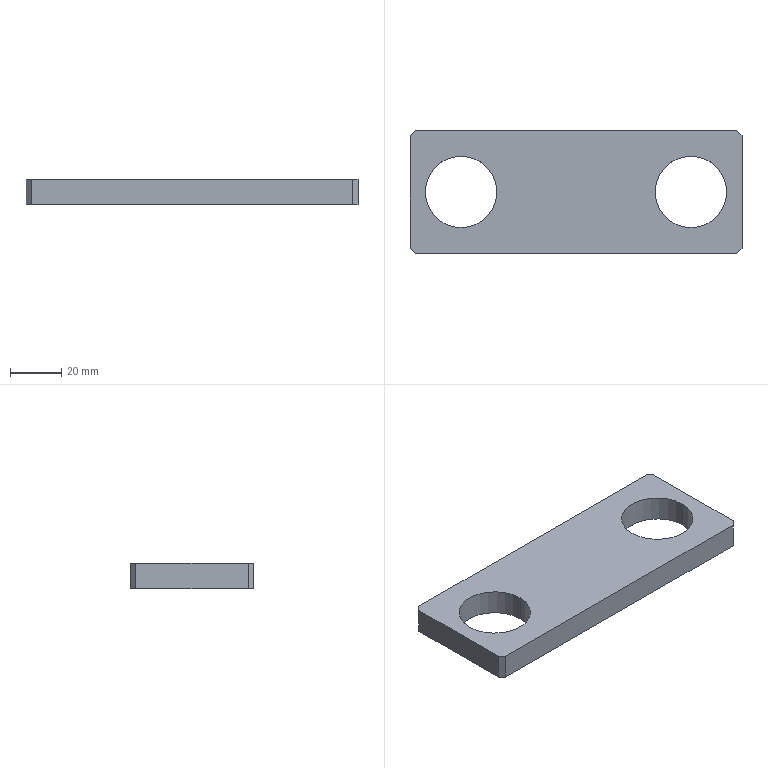Part | STEP file | Linear support fixing plate | 1 solid | 14 faces | box 130 x 48 x 10 mm | volume 50005 mm3 | plane 10 | cylinder 4 | commonest cylinder face diameters 28 x4
STEP:
#1=CARTESIAN_POINT('',(0.,0.,0.));
#2=DIRECTION('',(0.,0.,1.));
#3=DIRECTION('',(1.,0.,0.));
#4=AXIS2_PLACEMENT_3D('',#1,#2,#3);
#5=CARTESIAN_POINT('',(-31.,0.,0.));
#6=VERTEX_POINT('',#5);
#7=CARTESIAN_POINT('',(-31.,0.,10.));
#8=VERTEX_POINT('',#7);
#9=CARTESIAN_POINT('',(-31.,0.,0.));
#10=DIRECTION('',(0.,0.,1.));
#11=VECTOR('',#10,1.);
#12=LINE('',#9,#11);
#13=CARTESIAN_POINT('',(-45.,0.,0.));
#14=DIRECTION('',(0.,0.,1.));
#15=DIRECTION('',(1.,0.,0.));
#16=AXIS2_PLACEMENT_3D('',#13,#14,#15);
#17=CYLINDRICAL_SURFACE('',#16,14.);
#18=CARTESIAN_POINT('',(6.283,0.));
#19=DIRECTION('',(0.,1.));
#20=VECTOR('',#19,1.);
#21=LINE('',#18,#20);
#22=(GEOMETRIC_REPRESENTATION_CONTEXT(2)PARAMETRIC_REPRESENTATION_CONTEXT()REPRESENTATION_CONTEXT('',''));
#23=DEFINITIONAL_REPRESENTATION('',(#21),#22);
#24=PCURVE('',#17,#23);
#25=CARTESIAN_POINT('',(-45.,0.,0.));
#26=DIRECTION('',(0.,0.,1.));
#27=DIRECTION('',(1.,0.,0.));
#28=AXIS2_PLACEMENT_3D('',#25,#26,#27);
#29=CYLINDRICAL_SURFACE('',#28,14.);
#30=CARTESIAN_POINT('',(0.,0.));
#31=DIRECTION('',(0.,1.));
#32=VECTOR('',#31,1.);
#33=LINE('',#30,#32);
#34=(GEOMETRIC_REPRESENTATION_CONTEXT(2)PARAMETRIC_REPRESENTATION_CONTEXT()REPRESENTATION_CONTEXT('',''));
#35=DEFINITIONAL_REPRESENTATION('',(#33),#34);
#36=PCURVE('',#29,#35);
#37=SURFACE_CURVE('',#12,(#24,#36),.PCURVE_S1.);
#38=EDGE_CURVE('',#6,#8,#37,.T.);
#39=ORIENTED_EDGE('',*,*,#38,.T.);
#40=CARTESIAN_POINT('',(-59.,0.,10.));
#41=VERTEX_POINT('',#40);
#42=CARTESIAN_POINT('',(-45.,0.,10.));
#43=DIRECTION('',(0.,0.,-1.));
#44=DIRECTION('',(1.,0.,0.));
#45=AXIS2_PLACEMENT_3D('',#42,#43,#44);
#46=CIRCLE('',#45,14.);
#47=CARTESIAN_POINT('',(6.283,10.));
#48=DIRECTION('',(-1.,0.));
#49=VECTOR('',#48,1.);
#50=LINE('',#47,#49);
#51=(GEOMETRIC_REPRESENTATION_CONTEXT(2)PARAMETRIC_REPRESENTATION_CONTEXT()REPRESENTATION_CONTEXT('',''));
#52=DEFINITIONAL_REPRESENTATION('',(#50),#51);
#53=PCURVE('',#17,#52);
#54=CARTESIAN_POINT('',(0.,0.,10.));
#55=DIRECTION('',(0.,0.,1.));
#56=DIRECTION('',(1.,0.,0.));
#57=AXIS2_PLACEMENT_3D('',#54,#55,#56);
#58=PLANE('',#57);
#59=CARTESIAN_POINT('',(-31.,0.));
#60=CARTESIAN_POINT('',(-31.,-24.249));
#61=CARTESIAN_POINT('',(-52.,-12.124));
#62=CARTESIAN_POINT('',(-73.,0.));
#63=CARTESIAN_POINT('',(-52.,12.124));
#64=CARTESIAN_POINT('',(-31.,24.249));
#65=CARTESIAN_POINT('',(-31.,0.));
#66=(BOUNDED_CURVE()B_SPLINE_CURVE(2,(#59,#60,#61,#62,#63,#64,#65),.UNSPECIFIED.,.T.,.F.)B_SPLINE_CURVE_WITH_KNOTS((1,2,2,2,2,1),(-2.094,0.,2.094,4.189,6.283,8.378),.UNSPECIFIED.)CURVE()GEOMETRIC_REPRESENTATION_ITEM()RATIONAL_B_SPLINE_CURVE((1.,0.5,1.,0.5,1.,0.5,1.))REPRESENTATION_ITEM(''));
#67=(GEOMETRIC_REPRESENTATION_CONTEXT(2)PARAMETRIC_REPRESENTATION_CONTEXT()REPRESENTATION_CONTEXT('',''));
#68=DEFINITIONAL_REPRESENTATION('',(#66),#67);
#69=PCURVE('',#58,#68);
#70=SURFACE_CURVE('',#46,(#53,#69),.PCURVE_S1.);
#71=EDGE_CURVE('',#8,#41,#70,.T.);
#72=ORIENTED_EDGE('',*,*,#71,.T.);
#73=CARTESIAN_POINT('',(-59.,0.,0.));
#74=VERTEX_POINT('',#73);
#75=CARTESIAN_POINT('',(-59.,0.,0.));
#76=DIRECTION('',(0.,0.,1.));
#77=VECTOR('',#76,1.);
#78=LINE('',#75,#77);
#79=CARTESIAN_POINT('',(3.142,0.));
#80=DIRECTION('',(0.,1.));
#81=VECTOR('',#80,1.);
#82=LINE('',#79,#81);
#83=(GEOMETRIC_REPRESENTATION_CONTEXT(2)PARAMETRIC_REPRESENTATION_CONTEXT()REPRESENTATION_CONTEXT('',''));
#84=DEFINITIONAL_REPRESENTATION('',(#82),#83);
#85=PCURVE('',#17,#84);
#86=CARTESIAN_POINT('',(3.142,0.));
#87=DIRECTION('',(0.,1.));
#88=VECTOR('',#87,1.);
#89=LINE('',#86,#88);
#90=(GEOMETRIC_REPRESENTATION_CONTEXT(2)PARAMETRIC_REPRESENTATION_CONTEXT()REPRESENTATION_CONTEXT('',''));
#91=DEFINITIONAL_REPRESENTATION('',(#89),#90);
#92=PCURVE('',#29,#91);
#93=SURFACE_CURVE('',#78,(#85,#92),.PCURVE_S1.);
#94=EDGE_CURVE('',#74,#41,#93,.T.);
#95=ORIENTED_EDGE('',*,*,#94,.F.);
#96=CARTESIAN_POINT('',(-45.,0.,0.));
#97=DIRECTION('',(0.,0.,-1.));
#98=DIRECTION('',(1.,0.,0.));
#99=AXIS2_PLACEMENT_3D('',#96,#97,#98);
#100=CIRCLE('',#99,14.);
#101=CARTESIAN_POINT('',(6.283,0.));
#102=DIRECTION('',(-1.,0.));
#103=VECTOR('',#102,1.);
#104=LINE('',#101,#103);
#105=(GEOMETRIC_REPRESENTATION_CONTEXT(2)PARAMETRIC_REPRESENTATION_CONTEXT()REPRESENTATION_CONTEXT('',''));
#106=DEFINITIONAL_REPRESENTATION('',(#104),#105);
#107=PCURVE('',#17,#106);
#108=CARTESIAN_POINT('',(0.,0.,0.));
#109=DIRECTION('',(0.,0.,1.));
#110=DIRECTION('',(1.,0.,0.));
#111=AXIS2_PLACEMENT_3D('',#108,#109,#110);
#112=PLANE('',#111);
#113=CARTESIAN_POINT('',(-31.,0.));
#114=CARTESIAN_POINT('',(-31.,-24.249));
#115=CARTESIAN_POINT('',(-52.,-12.124));
#116=CARTESIAN_POINT('',(-73.,0.));
#117=CARTESIAN_POINT('',(-52.,12.124));
#118=CARTESIAN_POINT('',(-31.,24.249));
#119=CARTESIAN_POINT('',(-31.,0.));
#120=(BOUNDED_CURVE()B_SPLINE_CURVE(2,(#113,#114,#115,#116,#117,#118,#119),.UNSPECIFIED.,.T.,.F.)B_SPLINE_CURVE_WITH_KNOTS((1,2,2,2,2,1),(-2.094,0.,2.094,4.189,6.283,8.378),.UNSPECIFIED.)CURVE()GEOMETRIC_REPRESENTATION_ITEM()RATIONAL_B_SPLINE_CURVE((1.,0.5,1.,0.5,1.,0.5,1.))REPRESENTATION_ITEM(''));
#121=(GEOMETRIC_REPRESENTATION_CONTEXT(2)PARAMETRIC_REPRESENTATION_CONTEXT()REPRESENTATION_CONTEXT('',''));
#122=DEFINITIONAL_REPRESENTATION('',(#120),#121);
#123=PCURVE('',#112,#122);
#124=SURFACE_CURVE('',#100,(#107,#123),.PCURVE_S1.);
#125=EDGE_CURVE('',#6,#74,#124,.T.);
#126=ORIENTED_EDGE('',*,*,#125,.F.);
#127=EDGE_LOOP('',(#39,#72,#95,#126));
#128=FACE_BOUND('',#127,.F.);
#129=ADVANCED_FACE('',(#128),#17,.F.);
#130=CARTESIAN_POINT('',(59.,0.,0.));
#131=VERTEX_POINT('',#130);
#132=CARTESIAN_POINT('',(59.,0.,10.));
#133=VERTEX_POINT('',#132);
#134=CARTESIAN_POINT('',(59.,0.,0.));
#135=DIRECTION('',(0.,0.,1.));
#136=VECTOR('',#135,1.);
#137=LINE('',#134,#136);
#138=CARTESIAN_POINT('',(45.,0.,0.));
#139=DIRECTION('',(0.,0.,1.));
#140=DIRECTION('',(1.,0.,0.));
#141=AXIS2_PLACEMENT_3D('',#138,#139,#140);
#142=CYLINDRICAL_SURFACE('',#141,14.);
#143=CARTESIAN_POINT('',(6.283,0.));
#144=DIRECTION('',(0.,1.));
#145=VECTOR('',#144,1.);
#146=LINE('',#143,#145);
#147=(GEOMETRIC_REPRESENTATION_CONTEXT(2)PARAMETRIC_REPRESENTATION_CONTEXT()REPRESENTATION_CONTEXT('',''));
#148=DEFINITIONAL_REPRESENTATION('',(#146),#147);
#149=PCURVE('',#142,#148);
#150=CARTESIAN_POINT('',(45.,0.,0.));
#151=DIRECTION('',(0.,0.,1.));
#152=DIRECTION('',(1.,0.,0.));
#153=AXIS2_PLACEMENT_3D('',#150,#151,#152);
#154=CYLINDRICAL_SURFACE('',#153,14.);
#155=CARTESIAN_POINT('',(0.,0.));
#156=DIRECTION('',(0.,1.));
#157=VECTOR('',#156,1.);
#158=LINE('',#155,#157);
#159=(GEOMETRIC_REPRESENTATION_CONTEXT(2)PARAMETRIC_REPRESENTATION_CONTEXT()REPRESENTATION_CONTEXT('',''));
#160=DEFINITIONAL_REPRESENTATION('',(#158),#159);
#161=PCURVE('',#154,#160);
#162=SURFACE_CURVE('',#137,(#149,#161),.PCURVE_S1.);
#163=EDGE_CURVE('',#131,#133,#162,.T.);
#164=ORIENTED_EDGE('',*,*,#163,.T.);
#165=CARTESIAN_POINT('',(31.,0.,10.));
#166=VERTEX_POINT('',#165);
#167=CARTESIAN_POINT('',(45.,0.,10.));
#168=DIRECTION('',(0.,0.,-1.));
#169=DIRECTION('',(1.,0.,0.));
#170=AXIS2_PLACEMENT_3D('',#167,#168,#169);
#171=CIRCLE('',#170,14.);
#172=CARTESIAN_POINT('',(6.283,10.));
#173=DIRECTION('',(-1.,0.));
#174=VECTOR('',#173,1.);
#175=LINE('',#172,#174);
#176=(GEOMETRIC_REPRESENTATION_CONTEXT(2)PARAMETRIC_REPRESENTATION_CONTEXT()REPRESENTATION_CONTEXT('',''));
#177=DEFINITIONAL_REPRESENTATION('',(#175),#176);
#178=PCURVE('',#142,#177);
#179=CARTESIAN_POINT('',(59.,0.));
#180=CARTESIAN_POINT('',(59.,-24.249));
#181=CARTESIAN_POINT('',(38.,-12.124));
#182=CARTESIAN_POINT('',(17.,0.));
#183=CARTESIAN_POINT('',(38.,12.124));
#184=CARTESIAN_POINT('',(59.,24.249));
#185=CARTESIAN_POINT('',(59.,0.));
#186=(BOUNDED_CURVE()B_SPLINE_CURVE(2,(#179,#180,#181,#182,#183,#184,#185),.UNSPECIFIED.,.T.,.F.)B_SPLINE_CURVE_WITH_KNOTS((1,2,2,2,2,1),(-2.094,0.,2.094,4.189,6.283,8.378),.UNSPECIFIED.)CURVE()GEOMETRIC_REPRESENTATION_ITEM()RATIONAL_B_SPLINE_CURVE((1.,0.5,1.,0.5,1.,0.5,1.))REPRESENTATION_ITEM(''));
#187=(GEOMETRIC_REPRESENTATION_CONTEXT(2)PARAMETRIC_REPRESENTATION_CONTEXT()REPRESENTATION_CONTEXT('',''));
#188=DEFINITIONAL_REPRESENTATION('',(#186),#187);
#189=PCURVE('',#58,#188);
#190=SURFACE_CURVE('',#171,(#178,#189),.PCURVE_S1.);
#191=EDGE_CURVE('',#133,#166,#190,.T.);
#192=ORIENTED_EDGE('',*,*,#191,.T.);
#193=CARTESIAN_POINT('',(31.,0.,0.));
#194=VERTEX_POINT('',#193);
#195=CARTESIAN_POINT('',(31.,0.,0.));
#196=DIRECTION('',(0.,0.,1.));
#197=VECTOR('',#196,1.);
#198=LINE('',#195,#197);
#199=CARTESIAN_POINT('',(3.142,0.));
#200=DIRECTION('',(0.,1.));
#201=VECTOR('',#200,1.);
#202=LINE('',#199,#201);
#203=(GEOMETRIC_REPRESENTATION_CONTEXT(2)PARAMETRIC_REPRESENTATION_CONTEXT()REPRESENTATION_CONTEXT('',''));
#204=DEFINITIONAL_REPRESENTATION('',(#202),#203);
#205=PCURVE('',#142,#204);
#206=CARTESIAN_POINT('',(3.142,0.));
#207=DIRECTION('',(0.,1.));
#208=VECTOR('',#207,1.);
#209=LINE('',#206,#208);
#210=(GEOMETRIC_REPRESENTATION_CONTEXT(2)PARAMETRIC_REPRESENTATION_CONTEXT()REPRESENTATION_CONTEXT('',''));
#211=DEFINITIONAL_REPRESENTATION('',(#209),#210);
#212=PCURVE('',#154,#211);
#213=SURFACE_CURVE('',#198,(#205,#212),.PCURVE_S1.);
#214=EDGE_CURVE('',#194,#166,#213,.T.);
#215=ORIENTED_EDGE('',*,*,#214,.F.);
#216=CARTESIAN_POINT('',(45.,0.,0.));
#217=DIRECTION('',(0.,0.,-1.));
#218=DIRECTION('',(1.,0.,0.));
#219=AXIS2_PLACEMENT_3D('',#216,#217,#218);
#220=CIRCLE('',#219,14.);
#221=CARTESIAN_POINT('',(6.283,0.));
#222=DIRECTION('',(-1.,0.));
#223=VECTOR('',#222,1.);
#224=LINE('',#221,#223);
#225=(GEOMETRIC_REPRESENTATION_CONTEXT(2)PARAMETRIC_REPRESENTATION_CONTEXT()REPRESENTATION_CONTEXT('',''));
#226=DEFINITIONAL_REPRESENTATION('',(#224),#225);
#227=PCURVE('',#142,#226);
#228=CARTESIAN_POINT('',(59.,0.));
#229=CARTESIAN_POINT('',(59.,-24.249));
#230=CARTESIAN_POINT('',(38.,-12.124));
#231=CARTESIAN_POINT('',(17.,0.));
#232=CARTESIAN_POINT('',(38.,12.124));
#233=CARTESIAN_POINT('',(59.,24.249));
#234=CARTESIAN_POINT('',(59.,0.));
#235=(BOUNDED_CURVE()B_SPLINE_CURVE(2,(#228,#229,#230,#231,#232,#233,#234),.UNSPECIFIED.,.T.,.F.)B_SPLINE_CURVE_WITH_KNOTS((1,2,2,2,2,1),(-2.094,0.,2.094,4.189,6.283,8.378),.UNSPECIFIED.)CURVE()GEOMETRIC_REPRESENTATION_ITEM()RATIONAL_B_SPLINE_CURVE((1.,0.5,1.,0.5,1.,0.5,1.))REPRESENTATION_ITEM(''));
#236=(GEOMETRIC_REPRESENTATION_CONTEXT(2)PARAMETRIC_REPRESENTATION_CONTEXT()REPRESENTATION_CONTEXT('',''));
#237=DEFINITIONAL_REPRESENTATION('',(#235),#236);
#238=PCURVE('',#112,#237);
#239=SURFACE_CURVE('',#220,(#227,#238),.PCURVE_S1.);
#240=EDGE_CURVE('',#131,#194,#239,.T.);
#241=ORIENTED_EDGE('',*,*,#240,.F.);
#242=EDGE_LOOP('',(#164,#192,#215,#241));
#243=FACE_BOUND('',#242,.F.);
#244=ADVANCED_FACE('',(#243),#142,.F.);
#245=CARTESIAN_POINT('',(-63.,24.,0.));
#246=VERTEX_POINT('',#245);
#247=CARTESIAN_POINT('',(-65.,22.,0.));
#248=VERTEX_POINT('',#247);
#249=CARTESIAN_POINT('',(-63.,24.,0.));
#250=DIRECTION('',(-0.7071,-0.7071,0.));
#251=VECTOR('',#250,1.);
#252=LINE('',#249,#251);
#253=CARTESIAN_POINT('',(-63.,24.));
#254=DIRECTION('',(-0.7071,-0.7071));
#255=VECTOR('',#254,1.);
#256=LINE('',#253,#255);
#257=(GEOMETRIC_REPRESENTATION_CONTEXT(2)PARAMETRIC_REPRESENTATION_CONTEXT()REPRESENTATION_CONTEXT('',''));
#258=DEFINITIONAL_REPRESENTATION('',(#256),#257);
#259=PCURVE('',#112,#258);
#260=CARTESIAN_POINT('',(-65.,22.,10.));
#261=DIRECTION('',(0.7071,-0.7071,0.));
#262=DIRECTION('',(0.7071,0.7071,0.));
#263=AXIS2_PLACEMENT_3D('',#260,#261,#262);
#264=PLANE('',#263);
#265=CARTESIAN_POINT('',(2.828,-10.));
#266=DIRECTION('',(-1.,0.));
#267=VECTOR('',#266,1.);
#268=LINE('',#265,#267);
#269=(GEOMETRIC_REPRESENTATION_CONTEXT(2)PARAMETRIC_REPRESENTATION_CONTEXT()REPRESENTATION_CONTEXT('',''));
#270=DEFINITIONAL_REPRESENTATION('',(#268),#269);
#271=PCURVE('',#264,#270);
#272=SURFACE_CURVE('',#252,(#259,#271),.PCURVE_S1.);
#273=EDGE_CURVE('',#246,#248,#272,.T.);
#274=ORIENTED_EDGE('',*,*,#273,.F.);
#275=CARTESIAN_POINT('',(63.,24.,0.));
#276=VERTEX_POINT('',#275);
#277=CARTESIAN_POINT('',(0.,24.,0.));
#278=DIRECTION('',(-1.,0.,0.));
#279=VECTOR('',#278,1.);
#280=LINE('',#277,#279);
#281=CARTESIAN_POINT('',(0.,24.));
#282=DIRECTION('',(-1.,0.));
#283=VECTOR('',#282,1.);
#284=LINE('',#281,#283);
#285=(GEOMETRIC_REPRESENTATION_CONTEXT(2)PARAMETRIC_REPRESENTATION_CONTEXT()REPRESENTATION_CONTEXT('',''));
#286=DEFINITIONAL_REPRESENTATION('',(#284),#285);
#287=PCURVE('',#112,#286);
#288=CARTESIAN_POINT('',(-65.,24.,10.));
#289=DIRECTION('',(0.,-1.,0.));
#290=DIRECTION('',(0.,0.,-1.));
#291=AXIS2_PLACEMENT_3D('',#288,#289,#290);
#292=PLANE('',#291);
#293=CARTESIAN_POINT('',(10.,65.));
#294=DIRECTION('',(0.,-1.));
#295=VECTOR('',#294,1.);
#296=LINE('',#293,#295);
#297=(GEOMETRIC_REPRESENTATION_CONTEXT(2)PARAMETRIC_REPRESENTATION_CONTEXT()REPRESENTATION_CONTEXT('',''));
#298=DEFINITIONAL_REPRESENTATION('',(#296),#297);
#299=PCURVE('',#292,#298);
#300=SURFACE_CURVE('',#280,(#287,#299),.PCURVE_S1.);
#301=EDGE_CURVE('',#276,#246,#300,.T.);
#302=ORIENTED_EDGE('',*,*,#301,.F.);
#303=CARTESIAN_POINT('',(65.,22.,0.));
#304=VERTEX_POINT('',#303);
#305=CARTESIAN_POINT('',(65.,22.,0.));
#306=DIRECTION('',(-0.7071,0.7071,0.));
#307=VECTOR('',#306,1.);
#308=LINE('',#305,#307);
#309=CARTESIAN_POINT('',(65.,22.));
#310=DIRECTION('',(-0.7071,0.7071));
#311=VECTOR('',#310,1.);
#312=LINE('',#309,#311);
#313=(GEOMETRIC_REPRESENTATION_CONTEXT(2)PARAMETRIC_REPRESENTATION_CONTEXT()REPRESENTATION_CONTEXT('',''));
#314=DEFINITIONAL_REPRESENTATION('',(#312),#313);
#315=PCURVE('',#112,#314);
#316=CARTESIAN_POINT('',(63.,24.,10.));
#317=DIRECTION('',(-0.7071,-0.7071,0.));
#318=DIRECTION('',(0.7071,-0.7071,0.));
#319=AXIS2_PLACEMENT_3D('',#316,#317,#318);
#320=PLANE('',#319);
#321=CARTESIAN_POINT('',(2.828,-10.));
#322=DIRECTION('',(-1.,0.));
#323=VECTOR('',#322,1.);
#324=LINE('',#321,#323);
#325=(GEOMETRIC_REPRESENTATION_CONTEXT(2)PARAMETRIC_REPRESENTATION_CONTEXT()REPRESENTATION_CONTEXT('',''));
#326=DEFINITIONAL_REPRESENTATION('',(#324),#325);
#327=PCURVE('',#320,#326);
#328=SURFACE_CURVE('',#308,(#315,#327),.PCURVE_S1.);
#329=EDGE_CURVE('',#304,#276,#328,.T.);
#330=ORIENTED_EDGE('',*,*,#329,.F.);
#331=CARTESIAN_POINT('',(65.,-22.,0.));
#332=VERTEX_POINT('',#331);
#333=CARTESIAN_POINT('',(65.,0.,0.));
#334=DIRECTION('',(0.,1.,0.));
#335=VECTOR('',#334,1.);
#336=LINE('',#333,#335);
#337=CARTESIAN_POINT('',(65.,0.));
#338=DIRECTION('',(0.,1.));
#339=VECTOR('',#338,1.);
#340=LINE('',#337,#339);
#341=(GEOMETRIC_REPRESENTATION_CONTEXT(2)PARAMETRIC_REPRESENTATION_CONTEXT()REPRESENTATION_CONTEXT('',''));
#342=DEFINITIONAL_REPRESENTATION('',(#340),#341);
#343=PCURVE('',#112,#342);
#344=CARTESIAN_POINT('',(65.,24.,10.));
#345=DIRECTION('',(-1.,0.,0.));
#346=DIRECTION('',(0.,0.,1.));
#347=AXIS2_PLACEMENT_3D('',#344,#345,#346);
#348=PLANE('',#347);
#349=CARTESIAN_POINT('',(-10.,-24.));
#350=DIRECTION('',(0.,1.));
#351=VECTOR('',#350,1.);
#352=LINE('',#349,#351);
#353=(GEOMETRIC_REPRESENTATION_CONTEXT(2)PARAMETRIC_REPRESENTATION_CONTEXT()REPRESENTATION_CONTEXT('',''));
#354=DEFINITIONAL_REPRESENTATION('',(#352),#353);
#355=PCURVE('',#348,#354);
#356=SURFACE_CURVE('',#336,(#343,#355),.PCURVE_S1.);
#357=EDGE_CURVE('',#332,#304,#356,.T.);
#358=ORIENTED_EDGE('',*,*,#357,.F.);
#359=CARTESIAN_POINT('',(63.,-24.,0.));
#360=VERTEX_POINT('',#359);
#361=CARTESIAN_POINT('',(63.,-24.,0.));
#362=DIRECTION('',(0.7071,0.7071,0.));
#363=VECTOR('',#362,1.);
#364=LINE('',#361,#363);
#365=CARTESIAN_POINT('',(63.,-24.));
#366=DIRECTION('',(0.7071,0.7071));
#367=VECTOR('',#366,1.);
#368=LINE('',#365,#367);
#369=(GEOMETRIC_REPRESENTATION_CONTEXT(2)PARAMETRIC_REPRESENTATION_CONTEXT()REPRESENTATION_CONTEXT('',''));
#370=DEFINITIONAL_REPRESENTATION('',(#368),#369);
#371=PCURVE('',#112,#370);
#372=CARTESIAN_POINT('',(65.,-22.,10.));
#373=DIRECTION('',(-0.7071,0.7071,0.));
#374=DIRECTION('',(-0.7071,-0.7071,0.));
#375=AXIS2_PLACEMENT_3D('',#372,#373,#374);
#376=PLANE('',#375);
#377=CARTESIAN_POINT('',(2.828,-10.));
#378=DIRECTION('',(-1.,0.));
#379=VECTOR('',#378,1.);
#380=LINE('',#377,#379);
#381=(GEOMETRIC_REPRESENTATION_CONTEXT(2)PARAMETRIC_REPRESENTATION_CONTEXT()REPRESENTATION_CONTEXT('',''));
#382=DEFINITIONAL_REPRESENTATION('',(#380),#381);
#383=PCURVE('',#376,#382);
#384=SURFACE_CURVE('',#364,(#371,#383),.PCURVE_S1.);
#385=EDGE_CURVE('',#360,#332,#384,.T.);
#386=ORIENTED_EDGE('',*,*,#385,.F.);
#387=CARTESIAN_POINT('',(-63.,-24.,0.));
#388=VERTEX_POINT('',#387);
#389=CARTESIAN_POINT('',(0.,-24.,0.));
#390=DIRECTION('',(1.,0.,0.));
#391=VECTOR('',#390,1.);
#392=LINE('',#389,#391);
#393=CARTESIAN_POINT('',(0.,-24.));
#394=DIRECTION('',(1.,0.));
#395=VECTOR('',#394,1.);
#396=LINE('',#393,#395);
#397=(GEOMETRIC_REPRESENTATION_CONTEXT(2)PARAMETRIC_REPRESENTATION_CONTEXT()REPRESENTATION_CONTEXT('',''));
#398=DEFINITIONAL_REPRESENTATION('',(#396),#397);
#399=PCURVE('',#112,#398);
#400=CARTESIAN_POINT('',(-65.,-24.,10.));
#401=DIRECTION('',(0.,1.,0.));
#402=DIRECTION('',(0.,0.,1.));
#403=AXIS2_PLACEMENT_3D('',#400,#401,#402);
#404=PLANE('',#403);
#405=CARTESIAN_POINT('',(-10.,65.));
#406=DIRECTION('',(0.,1.));
#407=VECTOR('',#406,1.);
#408=LINE('',#405,#407);
#409=(GEOMETRIC_REPRESENTATION_CONTEXT(2)PARAMETRIC_REPRESENTATION_CONTEXT()REPRESENTATION_CONTEXT('',''));
#410=DEFINITIONAL_REPRESENTATION('',(#408),#409);
#411=PCURVE('',#404,#410);
#412=SURFACE_CURVE('',#392,(#399,#411),.PCURVE_S1.);
#413=EDGE_CURVE('',#388,#360,#412,.T.);
#414=ORIENTED_EDGE('',*,*,#413,.F.);
#415=CARTESIAN_POINT('',(-65.,-22.,0.));
#416=VERTEX_POINT('',#415);
#417=CARTESIAN_POINT('',(-65.,-22.,0.));
#418=DIRECTION('',(0.7071,-0.7071,0.));
#419=VECTOR('',#418,1.);
#420=LINE('',#417,#419);
#421=CARTESIAN_POINT('',(-65.,-22.));
#422=DIRECTION('',(0.7071,-0.7071));
#423=VECTOR('',#422,1.);
#424=LINE('',#421,#423);
#425=(GEOMETRIC_REPRESENTATION_CONTEXT(2)PARAMETRIC_REPRESENTATION_CONTEXT()REPRESENTATION_CONTEXT('',''));
#426=DEFINITIONAL_REPRESENTATION('',(#424),#425);
#427=PCURVE('',#112,#426);
#428=CARTESIAN_POINT('',(-63.,-24.,10.));
#429=DIRECTION('',(0.7071,0.7071,0.));
#430=DIRECTION('',(-0.7071,0.7071,0.));
#431=AXIS2_PLACEMENT_3D('',#428,#429,#430);
#432=PLANE('',#431);
#433=CARTESIAN_POINT('',(2.828,-10.));
#434=DIRECTION('',(-1.,0.));
#435=VECTOR('',#434,1.);
#436=LINE('',#433,#435);
#437=(GEOMETRIC_REPRESENTATION_CONTEXT(2)PARAMETRIC_REPRESENTATION_CONTEXT()REPRESENTATION_CONTEXT('',''));
#438=DEFINITIONAL_REPRESENTATION('',(#436),#437);
#439=PCURVE('',#432,#438);
#440=SURFACE_CURVE('',#420,(#427,#439),.PCURVE_S1.);
#441=EDGE_CURVE('',#416,#388,#440,.T.);
#442=ORIENTED_EDGE('',*,*,#441,.F.);
#443=CARTESIAN_POINT('',(-65.,0.,0.));
#444=DIRECTION('',(0.,-1.,0.));
#445=VECTOR('',#444,1.);
#446=LINE('',#443,#445);
#447=CARTESIAN_POINT('',(-65.,0.));
#448=DIRECTION('',(0.,-1.));
#449=VECTOR('',#448,1.);
#450=LINE('',#447,#449);
#451=(GEOMETRIC_REPRESENTATION_CONTEXT(2)PARAMETRIC_REPRESENTATION_CONTEXT()REPRESENTATION_CONTEXT('',''));
#452=DEFINITIONAL_REPRESENTATION('',(#450),#451);
#453=PCURVE('',#112,#452);
#454=CARTESIAN_POINT('',(-65.,24.,10.));
#455=DIRECTION('',(1.,0.,0.));
#456=DIRECTION('',(0.,0.,-1.));
#457=AXIS2_PLACEMENT_3D('',#454,#455,#456);
#458=PLANE('',#457);
#459=CARTESIAN_POINT('',(10.,-24.));
#460=DIRECTION('',(0.,-1.));
#461=VECTOR('',#460,1.);
#462=LINE('',#459,#461);
#463=(GEOMETRIC_REPRESENTATION_CONTEXT(2)PARAMETRIC_REPRESENTATION_CONTEXT()REPRESENTATION_CONTEXT('',''));
#464=DEFINITIONAL_REPRESENTATION('',(#462),#463);
#465=PCURVE('',#458,#464);
#466=SURFACE_CURVE('',#446,(#453,#465),.PCURVE_S1.);
#467=EDGE_CURVE('',#248,#416,#466,.T.);
#468=ORIENTED_EDGE('',*,*,#467,.F.);
#469=EDGE_LOOP('',(#274,#302,#330,#358,#386,#414,#442,#468));
#470=FACE_BOUND('',#469,.T.);
#471=ORIENTED_EDGE('',*,*,#125,.F.);
#472=CARTESIAN_POINT('',(-45.,0.,0.));
#473=DIRECTION('',(0.,0.,-1.));
#474=DIRECTION('',(1.,0.,0.));
#475=AXIS2_PLACEMENT_3D('',#472,#473,#474);
#476=CIRCLE('',#475,14.);
#477=CARTESIAN_POINT('',(-31.,0.));
#478=CARTESIAN_POINT('',(-31.,-24.249));
#479=CARTESIAN_POINT('',(-52.,-12.124));
#480=CARTESIAN_POINT('',(-73.,0.));
#481=CARTESIAN_POINT('',(-52.,12.124));
#482=CARTESIAN_POINT('',(-31.,24.249));
#483=CARTESIAN_POINT('',(-31.,0.));
#484=(BOUNDED_CURVE()B_SPLINE_CURVE(2,(#477,#478,#479,#480,#481,#482,#483),.UNSPECIFIED.,.T.,.F.)B_SPLINE_CURVE_WITH_KNOTS((1,2,2,2,2,1),(-2.094,0.,2.094,4.189,6.283,8.378),.UNSPECIFIED.)CURVE()GEOMETRIC_REPRESENTATION_ITEM()RATIONAL_B_SPLINE_CURVE((1.,0.5,1.,0.5,1.,0.5,1.))REPRESENTATION_ITEM(''));
#485=(GEOMETRIC_REPRESENTATION_CONTEXT(2)PARAMETRIC_REPRESENTATION_CONTEXT()REPRESENTATION_CONTEXT('',''));
#486=DEFINITIONAL_REPRESENTATION('',(#484),#485);
#487=PCURVE('',#112,#486);
#488=CARTESIAN_POINT('',(6.283,0.));
#489=DIRECTION('',(-1.,0.));
#490=VECTOR('',#489,1.);
#491=LINE('',#488,#490);
#492=(GEOMETRIC_REPRESENTATION_CONTEXT(2)PARAMETRIC_REPRESENTATION_CONTEXT()REPRESENTATION_CONTEXT('',''));
#493=DEFINITIONAL_REPRESENTATION('',(#491),#492);
#494=PCURVE('',#29,#493);
#495=SURFACE_CURVE('',#476,(#487,#494),.PCURVE_S1.);
#496=EDGE_CURVE('',#74,#6,#495,.T.);
#497=ORIENTED_EDGE('',*,*,#496,.F.);
#498=EDGE_LOOP('',(#471,#497));
#499=FACE_BOUND('',#498,.T.);
#500=ORIENTED_EDGE('',*,*,#240,.F.);
#501=CARTESIAN_POINT('',(45.,0.,0.));
#502=DIRECTION('',(0.,0.,-1.));
#503=DIRECTION('',(1.,0.,0.));
#504=AXIS2_PLACEMENT_3D('',#501,#502,#503);
#505=CIRCLE('',#504,14.);
#506=CARTESIAN_POINT('',(59.,0.));
#507=CARTESIAN_POINT('',(59.,-24.249));
#508=CARTESIAN_POINT('',(38.,-12.124));
#509=CARTESIAN_POINT('',(17.,0.));
#510=CARTESIAN_POINT('',(38.,12.124));
#511=CARTESIAN_POINT('',(59.,24.249));
#512=CARTESIAN_POINT('',(59.,0.));
#513=(BOUNDED_CURVE()B_SPLINE_CURVE(2,(#506,#507,#508,#509,#510,#511,#512),.UNSPECIFIED.,.T.,.F.)B_SPLINE_CURVE_WITH_KNOTS((1,2,2,2,2,1),(-2.094,0.,2.094,4.189,6.283,8.378),.UNSPECIFIED.)CURVE()GEOMETRIC_REPRESENTATION_ITEM()RATIONAL_B_SPLINE_CURVE((1.,0.5,1.,0.5,1.,0.5,1.))REPRESENTATION_ITEM(''));
#514=(GEOMETRIC_REPRESENTATION_CONTEXT(2)PARAMETRIC_REPRESENTATION_CONTEXT()REPRESENTATION_CONTEXT('',''));
#515=DEFINITIONAL_REPRESENTATION('',(#513),#514);
#516=PCURVE('',#112,#515);
#517=CARTESIAN_POINT('',(6.283,0.));
#518=DIRECTION('',(-1.,0.));
#519=VECTOR('',#518,1.);
#520=LINE('',#517,#519);
#521=(GEOMETRIC_REPRESENTATION_CONTEXT(2)PARAMETRIC_REPRESENTATION_CONTEXT()REPRESENTATION_CONTEXT('',''));
#522=DEFINITIONAL_REPRESENTATION('',(#520),#521);
#523=PCURVE('',#154,#522);
#524=SURFACE_CURVE('',#505,(#516,#523),.PCURVE_S1.);
#525=EDGE_CURVE('',#194,#131,#524,.T.);
#526=ORIENTED_EDGE('',*,*,#525,.F.);
#527=EDGE_LOOP('',(#500,#526));
#528=FACE_BOUND('',#527,.T.);
#529=ADVANCED_FACE('',(#470,#499,#528),#112,.F.);
#530=CARTESIAN_POINT('',(-65.,22.,10.));
#531=VERTEX_POINT('',#530);
#532=CARTESIAN_POINT('',(-65.,22.,10.));
#533=DIRECTION('',(0.,0.,1.));
#534=VECTOR('',#533,1.);
#535=LINE('',#532,#534);
#536=CARTESIAN_POINT('',(0.,-2.));
#537=DIRECTION('',(-1.,0.));
#538=VECTOR('',#537,1.);
#539=LINE('',#536,#538);
#540=(GEOMETRIC_REPRESENTATION_CONTEXT(2)PARAMETRIC_REPRESENTATION_CONTEXT()REPRESENTATION_CONTEXT('',''));
#541=DEFINITIONAL_REPRESENTATION('',(#539),#540);
#542=PCURVE('',#458,#541);
#543=CARTESIAN_POINT('',(0.,0.));
#544=DIRECTION('',(0.,1.));
#545=VECTOR('',#544,1.);
#546=LINE('',#543,#545);
#547=(GEOMETRIC_REPRESENTATION_CONTEXT(2)PARAMETRIC_REPRESENTATION_CONTEXT()REPRESENTATION_CONTEXT('',''));
#548=DEFINITIONAL_REPRESENTATION('',(#546),#547);
#549=PCURVE('',#264,#548);
#550=SURFACE_CURVE('',#535,(#542,#549),.PCURVE_S1.);
#551=EDGE_CURVE('',#248,#531,#550,.T.);
#552=ORIENTED_EDGE('',*,*,#551,.F.);
#553=ORIENTED_EDGE('',*,*,#467,.T.);
#554=CARTESIAN_POINT('',(-65.,-22.,10.));
#555=VERTEX_POINT('',#554);
#556=CARTESIAN_POINT('',(-65.,-22.,10.));
#557=DIRECTION('',(0.,0.,-1.));
#558=VECTOR('',#557,1.);
#559=LINE('',#556,#558);
#560=CARTESIAN_POINT('',(0.,-46.));
#561=DIRECTION('',(1.,0.));
#562=VECTOR('',#561,1.);
#563=LINE('',#560,#562);
#564=(GEOMETRIC_REPRESENTATION_CONTEXT(2)PARAMETRIC_REPRESENTATION_CONTEXT()REPRESENTATION_CONTEXT('',''));
#565=DEFINITIONAL_REPRESENTATION('',(#563),#564);
#566=PCURVE('',#458,#565);
#567=CARTESIAN_POINT('',(2.828,0.));
#568=DIRECTION('',(0.,-1.));
#569=VECTOR('',#568,1.);
#570=LINE('',#567,#569);
#571=(GEOMETRIC_REPRESENTATION_CONTEXT(2)PARAMETRIC_REPRESENTATION_CONTEXT()REPRESENTATION_CONTEXT('',''));
#572=DEFINITIONAL_REPRESENTATION('',(#570),#571);
#573=PCURVE('',#432,#572);
#574=SURFACE_CURVE('',#559,(#566,#573),.PCURVE_S1.);
#575=EDGE_CURVE('',#555,#416,#574,.T.);
#576=ORIENTED_EDGE('',*,*,#575,.F.);
#577=CARTESIAN_POINT('',(-65.,24.,10.));
#578=DIRECTION('',(0.,-1.,0.));
#579=VECTOR('',#578,1.);
#580=LINE('',#577,#579);
#581=CARTESIAN_POINT('',(0.,0.));
#582=DIRECTION('',(0.,-1.));
#583=VECTOR('',#582,1.);
#584=LINE('',#581,#583);
#585=(GEOMETRIC_REPRESENTATION_CONTEXT(2)PARAMETRIC_REPRESENTATION_CONTEXT()REPRESENTATION_CONTEXT('',''));
#586=DEFINITIONAL_REPRESENTATION('',(#584),#585);
#587=PCURVE('',#458,#586);
#588=CARTESIAN_POINT('',(-65.,24.));
#589=DIRECTION('',(0.,-1.));
#590=VECTOR('',#589,1.);
#591=LINE('',#588,#590);
#592=(GEOMETRIC_REPRESENTATION_CONTEXT(2)PARAMETRIC_REPRESENTATION_CONTEXT()REPRESENTATION_CONTEXT('',''));
#593=DEFINITIONAL_REPRESENTATION('',(#591),#592);
#594=PCURVE('',#58,#593);
#595=SURFACE_CURVE('',#580,(#587,#594),.PCURVE_S1.);
#596=EDGE_CURVE('',#531,#555,#595,.T.);
#597=ORIENTED_EDGE('',*,*,#596,.F.);
#598=EDGE_LOOP('',(#552,#553,#576,#597));
#599=FACE_BOUND('',#598,.T.);
#600=ADVANCED_FACE('',(#599),#458,.F.);
#601=CARTESIAN_POINT('',(-63.,24.,10.));
#602=VERTEX_POINT('',#601);
#603=CARTESIAN_POINT('',(-63.,24.,10.));
#604=DIRECTION('',(0.,0.,1.));
#605=VECTOR('',#604,1.);
#606=LINE('',#603,#605);
#607=CARTESIAN_POINT('',(2.828,0.));
#608=DIRECTION('',(0.,1.));
#609=VECTOR('',#608,1.);
#610=LINE('',#607,#609);
#611=(GEOMETRIC_REPRESENTATION_CONTEXT(2)PARAMETRIC_REPRESENTATION_CONTEXT()REPRESENTATION_CONTEXT('',''));
#612=DEFINITIONAL_REPRESENTATION('',(#610),#611);
#613=PCURVE('',#264,#612);
#614=CARTESIAN_POINT('',(0.,2.));
#615=DIRECTION('',(-1.,0.));
#616=VECTOR('',#615,1.);
#617=LINE('',#614,#616);
#618=(GEOMETRIC_REPRESENTATION_CONTEXT(2)PARAMETRIC_REPRESENTATION_CONTEXT()REPRESENTATION_CONTEXT('',''));
#619=DEFINITIONAL_REPRESENTATION('',(#617),#618);
#620=PCURVE('',#292,#619);
#621=SURFACE_CURVE('',#606,(#613,#620),.PCURVE_S1.);
#622=EDGE_CURVE('',#246,#602,#621,.T.);
#623=ORIENTED_EDGE('',*,*,#622,.F.);
#624=ORIENTED_EDGE('',*,*,#273,.T.);
#625=ORIENTED_EDGE('',*,*,#551,.T.);
#626=CARTESIAN_POINT('',(-65.,22.,10.));
#627=DIRECTION('',(-0.7071,-0.7071,0.));
#628=VECTOR('',#627,1.);
#629=LINE('',#626,#628);
#630=CARTESIAN_POINT('',(0.,0.));
#631=DIRECTION('',(-1.,0.));
#632=VECTOR('',#631,1.);
#633=LINE('',#630,#632);
#634=(GEOMETRIC_REPRESENTATION_CONTEXT(2)PARAMETRIC_REPRESENTATION_CONTEXT()REPRESENTATION_CONTEXT('',''));
#635=DEFINITIONAL_REPRESENTATION('',(#633),#634);
#636=PCURVE('',#264,#635);
#637=CARTESIAN_POINT('',(-65.,22.));
#638=DIRECTION('',(-0.7071,-0.7071));
#639=VECTOR('',#638,1.);
#640=LINE('',#637,#639);
#641=(GEOMETRIC_REPRESENTATION_CONTEXT(2)PARAMETRIC_REPRESENTATION_CONTEXT()REPRESENTATION_CONTEXT('',''));
#642=DEFINITIONAL_REPRESENTATION('',(#640),#641);
#643=PCURVE('',#58,#642);
#644=SURFACE_CURVE('',#629,(#636,#643),.PCURVE_S1.);
#645=EDGE_CURVE('',#602,#531,#644,.T.);
#646=ORIENTED_EDGE('',*,*,#645,.F.);
#647=EDGE_LOOP('',(#623,#624,#625,#646));
#648=FACE_BOUND('',#647,.T.);
#649=ADVANCED_FACE('',(#648),#264,.F.);
#650=ORIENTED_EDGE('',*,*,#622,.T.);
#651=CARTESIAN_POINT('',(63.,24.,10.));
#652=VERTEX_POINT('',#651);
#653=CARTESIAN_POINT('',(-65.,24.,10.));
#654=DIRECTION('',(-1.,0.,0.));
#655=VECTOR('',#654,1.);
#656=LINE('',#653,#655);
#657=CARTESIAN_POINT('',(0.,0.));
#658=DIRECTION('',(0.,-1.));
#659=VECTOR('',#658,1.);
#660=LINE('',#657,#659);
#661=(GEOMETRIC_REPRESENTATION_CONTEXT(2)PARAMETRIC_REPRESENTATION_CONTEXT()REPRESENTATION_CONTEXT('',''));
#662=DEFINITIONAL_REPRESENTATION('',(#660),#661);
#663=PCURVE('',#292,#662);
#664=CARTESIAN_POINT('',(-65.,24.));
#665=DIRECTION('',(-1.,0.));
#666=VECTOR('',#665,1.);
#667=LINE('',#664,#666);
#668=(GEOMETRIC_REPRESENTATION_CONTEXT(2)PARAMETRIC_REPRESENTATION_CONTEXT()REPRESENTATION_CONTEXT('',''));
#669=DEFINITIONAL_REPRESENTATION('',(#667),#668);
#670=PCURVE('',#58,#669);
#671=SURFACE_CURVE('',#656,(#663,#670),.PCURVE_S1.);
#672=EDGE_CURVE('',#652,#602,#671,.T.);
#673=ORIENTED_EDGE('',*,*,#672,.F.);
#674=CARTESIAN_POINT('',(63.,24.,10.));
#675=DIRECTION('',(0.,0.,1.));
#676=VECTOR('',#675,1.);
#677=LINE('',#674,#676);
#678=CARTESIAN_POINT('',(0.,128.));
#679=DIRECTION('',(-1.,0.));
#680=VECTOR('',#679,1.);
#681=LINE('',#678,#680);
#682=(GEOMETRIC_REPRESENTATION_CONTEXT(2)PARAMETRIC_REPRESENTATION_CONTEXT()REPRESENTATION_CONTEXT('',''));
#683=DEFINITIONAL_REPRESENTATION('',(#681),#682);
#684=PCURVE('',#292,#683);
#685=CARTESIAN_POINT('',(0.,0.));
#686=DIRECTION('',(0.,1.));
#687=VECTOR('',#686,1.);
#688=LINE('',#685,#687);
#689=(GEOMETRIC_REPRESENTATION_CONTEXT(2)PARAMETRIC_REPRESENTATION_CONTEXT()REPRESENTATION_CONTEXT('',''));
#690=DEFINITIONAL_REPRESENTATION('',(#688),#689);
#691=PCURVE('',#320,#690);
#692=SURFACE_CURVE('',#677,(#684,#691),.PCURVE_S1.);
#693=EDGE_CURVE('',#276,#652,#692,.T.);
#694=ORIENTED_EDGE('',*,*,#693,.F.);
#695=ORIENTED_EDGE('',*,*,#301,.T.);
#696=EDGE_LOOP('',(#650,#673,#694,#695));
#697=FACE_BOUND('',#696,.T.);
#698=ADVANCED_FACE('',(#697),#292,.F.);
#699=CARTESIAN_POINT('',(65.,22.,10.));
#700=VERTEX_POINT('',#699);
#701=CARTESIAN_POINT('',(65.,22.,10.));
#702=DIRECTION('',(0.,0.,1.));
#703=VECTOR('',#702,1.);
#704=LINE('',#701,#703);
#705=CARTESIAN_POINT('',(2.828,0.));
#706=DIRECTION('',(0.,1.));
#707=VECTOR('',#706,1.);
#708=LINE('',#705,#707);
#709=(GEOMETRIC_REPRESENTATION_CONTEXT(2)PARAMETRIC_REPRESENTATION_CONTEXT()REPRESENTATION_CONTEXT('',''));
#710=DEFINITIONAL_REPRESENTATION('',(#708),#709);
#711=PCURVE('',#320,#710);
#712=CARTESIAN_POINT('',(0.,-2.));
#713=DIRECTION('',(1.,0.));
#714=VECTOR('',#713,1.);
#715=LINE('',#712,#714);
#716=(GEOMETRIC_REPRESENTATION_CONTEXT(2)PARAMETRIC_REPRESENTATION_CONTEXT()REPRESENTATION_CONTEXT('',''));
#717=DEFINITIONAL_REPRESENTATION('',(#715),#716);
#718=PCURVE('',#348,#717);
#719=SURFACE_CURVE('',#704,(#711,#718),.PCURVE_S1.);
#720=EDGE_CURVE('',#304,#700,#719,.T.);
#721=ORIENTED_EDGE('',*,*,#720,.F.);
#722=ORIENTED_EDGE('',*,*,#329,.T.);
#723=ORIENTED_EDGE('',*,*,#693,.T.);
#724=CARTESIAN_POINT('',(63.,24.,10.));
#725=DIRECTION('',(-0.7071,0.7071,0.));
#726=VECTOR('',#725,1.);
#727=LINE('',#724,#726);
#728=CARTESIAN_POINT('',(0.,0.));
#729=DIRECTION('',(-1.,0.));
#730=VECTOR('',#729,1.);
#731=LINE('',#728,#730);
#732=(GEOMETRIC_REPRESENTATION_CONTEXT(2)PARAMETRIC_REPRESENTATION_CONTEXT()REPRESENTATION_CONTEXT('',''));
#733=DEFINITIONAL_REPRESENTATION('',(#731),#732);
#734=PCURVE('',#320,#733);
#735=CARTESIAN_POINT('',(63.,24.));
#736=DIRECTION('',(-0.7071,0.7071));
#737=VECTOR('',#736,1.);
#738=LINE('',#735,#737);
#739=(GEOMETRIC_REPRESENTATION_CONTEXT(2)PARAMETRIC_REPRESENTATION_CONTEXT()REPRESENTATION_CONTEXT('',''));
#740=DEFINITIONAL_REPRESENTATION('',(#738),#739);
#741=PCURVE('',#58,#740);
#742=SURFACE_CURVE('',#727,(#734,#741),.PCURVE_S1.);
#743=EDGE_CURVE('',#700,#652,#742,.T.);
#744=ORIENTED_EDGE('',*,*,#743,.F.);
#745=EDGE_LOOP('',(#721,#722,#723,#744));
#746=FACE_BOUND('',#745,.T.);
#747=ADVANCED_FACE('',(#746),#320,.F.);
#748=ORIENTED_EDGE('',*,*,#720,.T.);
#749=CARTESIAN_POINT('',(65.,-22.,10.));
#750=VERTEX_POINT('',#749);
#751=CARTESIAN_POINT('',(65.,24.,10.));
#752=DIRECTION('',(0.,1.,0.));
#753=VECTOR('',#752,1.);
#754=LINE('',#751,#753);
#755=CARTESIAN_POINT('',(0.,0.));
#756=DIRECTION('',(0.,1.));
#757=VECTOR('',#756,1.);
#758=LINE('',#755,#757);
#759=(GEOMETRIC_REPRESENTATION_CONTEXT(2)PARAMETRIC_REPRESENTATION_CONTEXT()REPRESENTATION_CONTEXT('',''));
#760=DEFINITIONAL_REPRESENTATION('',(#758),#759);
#761=PCURVE('',#348,#760);
#762=CARTESIAN_POINT('',(65.,24.));
#763=DIRECTION('',(0.,1.));
#764=VECTOR('',#763,1.);
#765=LINE('',#762,#764);
#766=(GEOMETRIC_REPRESENTATION_CONTEXT(2)PARAMETRIC_REPRESENTATION_CONTEXT()REPRESENTATION_CONTEXT('',''));
#767=DEFINITIONAL_REPRESENTATION('',(#765),#766);
#768=PCURVE('',#58,#767);
#769=SURFACE_CURVE('',#754,(#761,#768),.PCURVE_S1.);
#770=EDGE_CURVE('',#750,#700,#769,.T.);
#771=ORIENTED_EDGE('',*,*,#770,.F.);
#772=CARTESIAN_POINT('',(65.,-22.,10.));
#773=DIRECTION('',(0.,0.,1.));
#774=VECTOR('',#773,1.);
#775=LINE('',#772,#774);
#776=CARTESIAN_POINT('',(0.,-46.));
#777=DIRECTION('',(1.,0.));
#778=VECTOR('',#777,1.);
#779=LINE('',#776,#778);
#780=(GEOMETRIC_REPRESENTATION_CONTEXT(2)PARAMETRIC_REPRESENTATION_CONTEXT()REPRESENTATION_CONTEXT('',''));
#781=DEFINITIONAL_REPRESENTATION('',(#779),#780);
#782=PCURVE('',#348,#781);
#783=CARTESIAN_POINT('',(0.,0.));
#784=DIRECTION('',(0.,1.));
#785=VECTOR('',#784,1.);
#786=LINE('',#783,#785);
#787=(GEOMETRIC_REPRESENTATION_CONTEXT(2)PARAMETRIC_REPRESENTATION_CONTEXT()REPRESENTATION_CONTEXT('',''));
#788=DEFINITIONAL_REPRESENTATION('',(#786),#787);
#789=PCURVE('',#376,#788);
#790=SURFACE_CURVE('',#775,(#782,#789),.PCURVE_S1.);
#791=EDGE_CURVE('',#332,#750,#790,.T.);
#792=ORIENTED_EDGE('',*,*,#791,.F.);
#793=ORIENTED_EDGE('',*,*,#357,.T.);
#794=EDGE_LOOP('',(#748,#771,#792,#793));
#795=FACE_BOUND('',#794,.T.);
#796=ADVANCED_FACE('',(#795),#348,.F.);
#797=CARTESIAN_POINT('',(63.,-24.,10.));
#798=VERTEX_POINT('',#797);
#799=CARTESIAN_POINT('',(63.,-24.,10.));
#800=DIRECTION('',(0.,0.,1.));
#801=VECTOR('',#800,1.);
#802=LINE('',#799,#801);
#803=CARTESIAN_POINT('',(2.828,0.));
#804=DIRECTION('',(0.,1.));
#805=VECTOR('',#804,1.);
#806=LINE('',#803,#805);
#807=(GEOMETRIC_REPRESENTATION_CONTEXT(2)PARAMETRIC_REPRESENTATION_CONTEXT()REPRESENTATION_CONTEXT('',''));
#808=DEFINITIONAL_REPRESENTATION('',(#806),#807);
#809=PCURVE('',#376,#808);
#810=CARTESIAN_POINT('',(0.,128.));
#811=DIRECTION('',(1.,0.));
#812=VECTOR('',#811,1.);
#813=LINE('',#810,#812);
#814=(GEOMETRIC_REPRESENTATION_CONTEXT(2)PARAMETRIC_REPRESENTATION_CONTEXT()REPRESENTATION_CONTEXT('',''));
#815=DEFINITIONAL_REPRESENTATION('',(#813),#814);
#816=PCURVE('',#404,#815);
#817=SURFACE_CURVE('',#802,(#809,#816),.PCURVE_S1.);
#818=EDGE_CURVE('',#360,#798,#817,.T.);
#819=ORIENTED_EDGE('',*,*,#818,.F.);
#820=ORIENTED_EDGE('',*,*,#385,.T.);
#821=ORIENTED_EDGE('',*,*,#791,.T.);
#822=CARTESIAN_POINT('',(65.,-22.,10.));
#823=DIRECTION('',(0.7071,0.7071,0.));
#824=VECTOR('',#823,1.);
#825=LINE('',#822,#824);
#826=CARTESIAN_POINT('',(0.,0.));
#827=DIRECTION('',(-1.,0.));
#828=VECTOR('',#827,1.);
#829=LINE('',#826,#828);
#830=(GEOMETRIC_REPRESENTATION_CONTEXT(2)PARAMETRIC_REPRESENTATION_CONTEXT()REPRESENTATION_CONTEXT('',''));
#831=DEFINITIONAL_REPRESENTATION('',(#829),#830);
#832=PCURVE('',#376,#831);
#833=CARTESIAN_POINT('',(65.,-22.));
#834=DIRECTION('',(0.7071,0.7071));
#835=VECTOR('',#834,1.);
#836=LINE('',#833,#835);
#837=(GEOMETRIC_REPRESENTATION_CONTEXT(2)PARAMETRIC_REPRESENTATION_CONTEXT()REPRESENTATION_CONTEXT('',''));
#838=DEFINITIONAL_REPRESENTATION('',(#836),#837);
#839=PCURVE('',#58,#838);
#840=SURFACE_CURVE('',#825,(#832,#839),.PCURVE_S1.);
#841=EDGE_CURVE('',#798,#750,#840,.T.);
#842=ORIENTED_EDGE('',*,*,#841,.F.);
#843=EDGE_LOOP('',(#819,#820,#821,#842));
#844=FACE_BOUND('',#843,.T.);
#845=ADVANCED_FACE('',(#844),#376,.F.);
#846=CARTESIAN_POINT('',(-63.,-24.,10.));
#847=VERTEX_POINT('',#846);
#848=CARTESIAN_POINT('',(-63.,-24.,10.));
#849=DIRECTION('',(0.,0.,1.));
#850=VECTOR('',#849,1.);
#851=LINE('',#848,#850);
#852=CARTESIAN_POINT('',(0.,2.));
#853=DIRECTION('',(1.,0.));
#854=VECTOR('',#853,1.);
#855=LINE('',#852,#854);
#856=(GEOMETRIC_REPRESENTATION_CONTEXT(2)PARAMETRIC_REPRESENTATION_CONTEXT()REPRESENTATION_CONTEXT('',''));
#857=DEFINITIONAL_REPRESENTATION('',(#855),#856);
#858=PCURVE('',#404,#857);
#859=CARTESIAN_POINT('',(0.,0.));
#860=DIRECTION('',(0.,1.));
#861=VECTOR('',#860,1.);
#862=LINE('',#859,#861);
#863=(GEOMETRIC_REPRESENTATION_CONTEXT(2)PARAMETRIC_REPRESENTATION_CONTEXT()REPRESENTATION_CONTEXT('',''));
#864=DEFINITIONAL_REPRESENTATION('',(#862),#863);
#865=PCURVE('',#432,#864);
#866=SURFACE_CURVE('',#851,(#858,#865),.PCURVE_S1.);
#867=EDGE_CURVE('',#388,#847,#866,.T.);
#868=ORIENTED_EDGE('',*,*,#867,.F.);
#869=ORIENTED_EDGE('',*,*,#413,.T.);
#870=ORIENTED_EDGE('',*,*,#818,.T.);
#871=CARTESIAN_POINT('',(-65.,-24.,10.));
#872=DIRECTION('',(1.,0.,0.));
#873=VECTOR('',#872,1.);
#874=LINE('',#871,#873);
#875=CARTESIAN_POINT('',(0.,0.));
#876=DIRECTION('',(0.,1.));
#877=VECTOR('',#876,1.);
#878=LINE('',#875,#877);
#879=(GEOMETRIC_REPRESENTATION_CONTEXT(2)PARAMETRIC_REPRESENTATION_CONTEXT()REPRESENTATION_CONTEXT('',''));
#880=DEFINITIONAL_REPRESENTATION('',(#878),#879);
#881=PCURVE('',#404,#880);
#882=CARTESIAN_POINT('',(-65.,-24.));
#883=DIRECTION('',(1.,0.));
#884=VECTOR('',#883,1.);
#885=LINE('',#882,#884);
#886=(GEOMETRIC_REPRESENTATION_CONTEXT(2)PARAMETRIC_REPRESENTATION_CONTEXT()REPRESENTATION_CONTEXT('',''));
#887=DEFINITIONAL_REPRESENTATION('',(#885),#886);
#888=PCURVE('',#58,#887);
#889=SURFACE_CURVE('',#874,(#881,#888),.PCURVE_S1.);
#890=EDGE_CURVE('',#847,#798,#889,.T.);
#891=ORIENTED_EDGE('',*,*,#890,.F.);
#892=EDGE_LOOP('',(#868,#869,#870,#891));
#893=FACE_BOUND('',#892,.T.);
#894=ADVANCED_FACE('',(#893),#404,.F.);
#895=ORIENTED_EDGE('',*,*,#575,.T.);
#896=ORIENTED_EDGE('',*,*,#441,.T.);
#897=ORIENTED_EDGE('',*,*,#867,.T.);
#898=CARTESIAN_POINT('',(-63.,-24.,10.));
#899=DIRECTION('',(0.7071,-0.7071,0.));
#900=VECTOR('',#899,1.);
#901=LINE('',#898,#900);
#902=CARTESIAN_POINT('',(0.,0.));
#903=DIRECTION('',(-1.,0.));
#904=VECTOR('',#903,1.);
#905=LINE('',#902,#904);
#906=(GEOMETRIC_REPRESENTATION_CONTEXT(2)PARAMETRIC_REPRESENTATION_CONTEXT()REPRESENTATION_CONTEXT('',''));
#907=DEFINITIONAL_REPRESENTATION('',(#905),#906);
#908=PCURVE('',#432,#907);
#909=CARTESIAN_POINT('',(-63.,-24.));
#910=DIRECTION('',(0.7071,-0.7071));
#911=VECTOR('',#910,1.);
#912=LINE('',#909,#911);
#913=(GEOMETRIC_REPRESENTATION_CONTEXT(2)PARAMETRIC_REPRESENTATION_CONTEXT()REPRESENTATION_CONTEXT('',''));
#914=DEFINITIONAL_REPRESENTATION('',(#912),#913);
#915=PCURVE('',#58,#914);
#916=SURFACE_CURVE('',#901,(#908,#915),.PCURVE_S1.);
#917=EDGE_CURVE('',#555,#847,#916,.T.);
#918=ORIENTED_EDGE('',*,*,#917,.F.);
#919=EDGE_LOOP('',(#895,#896,#897,#918));
#920=FACE_BOUND('',#919,.T.);
#921=ADVANCED_FACE('',(#920),#432,.F.);
#922=CARTESIAN_POINT('',(-45.,0.,10.));
#923=DIRECTION('',(0.,0.,-1.));
#924=DIRECTION('',(1.,0.,0.));
#925=AXIS2_PLACEMENT_3D('',#922,#923,#924);
#926=CIRCLE('',#925,14.);
#927=CARTESIAN_POINT('',(6.283,10.));
#928=DIRECTION('',(-1.,0.));
#929=VECTOR('',#928,1.);
#930=LINE('',#927,#929);
#931=(GEOMETRIC_REPRESENTATION_CONTEXT(2)PARAMETRIC_REPRESENTATION_CONTEXT()REPRESENTATION_CONTEXT('',''));
#932=DEFINITIONAL_REPRESENTATION('',(#930),#931);
#933=PCURVE('',#29,#932);
#934=CARTESIAN_POINT('',(-31.,0.));
#935=CARTESIAN_POINT('',(-31.,-24.249));
#936=CARTESIAN_POINT('',(-52.,-12.124));
#937=CARTESIAN_POINT('',(-73.,0.));
#938=CARTESIAN_POINT('',(-52.,12.124));
#939=CARTESIAN_POINT('',(-31.,24.249));
#940=CARTESIAN_POINT('',(-31.,0.));
#941=(BOUNDED_CURVE()B_SPLINE_CURVE(2,(#934,#935,#936,#937,#938,#939,#940),.UNSPECIFIED.,.T.,.F.)B_SPLINE_CURVE_WITH_KNOTS((1,2,2,2,2,1),(-2.094,0.,2.094,4.189,6.283,8.378),.UNSPECIFIED.)CURVE()GEOMETRIC_REPRESENTATION_ITEM()RATIONAL_B_SPLINE_CURVE((1.,0.5,1.,0.5,1.,0.5,1.))REPRESENTATION_ITEM(''));
#942=(GEOMETRIC_REPRESENTATION_CONTEXT(2)PARAMETRIC_REPRESENTATION_CONTEXT()REPRESENTATION_CONTEXT('',''));
#943=DEFINITIONAL_REPRESENTATION('',(#941),#942);
#944=PCURVE('',#58,#943);
#945=SURFACE_CURVE('',#926,(#933,#944),.PCURVE_S1.);
#946=EDGE_CURVE('',#41,#8,#945,.T.);
#947=ORIENTED_EDGE('',*,*,#946,.T.);
#948=ORIENTED_EDGE('',*,*,#38,.F.);
#949=ORIENTED_EDGE('',*,*,#496,.F.);
#950=ORIENTED_EDGE('',*,*,#94,.T.);
#951=EDGE_LOOP('',(#947,#948,#949,#950));
#952=FACE_BOUND('',#951,.F.);
#953=ADVANCED_FACE('',(#952),#29,.F.);
#954=CARTESIAN_POINT('',(45.,0.,10.));
#955=DIRECTION('',(0.,0.,-1.));
#956=DIRECTION('',(1.,0.,0.));
#957=AXIS2_PLACEMENT_3D('',#954,#955,#956);
#958=CIRCLE('',#957,14.);
#959=CARTESIAN_POINT('',(6.283,10.));
#960=DIRECTION('',(-1.,0.));
#961=VECTOR('',#960,1.);
#962=LINE('',#959,#961);
#963=(GEOMETRIC_REPRESENTATION_CONTEXT(2)PARAMETRIC_REPRESENTATION_CONTEXT()REPRESENTATION_CONTEXT('',''));
#964=DEFINITIONAL_REPRESENTATION('',(#962),#963);
#965=PCURVE('',#154,#964);
#966=CARTESIAN_POINT('',(59.,0.));
#967=CARTESIAN_POINT('',(59.,-24.249));
#968=CARTESIAN_POINT('',(38.,-12.124));
#969=CARTESIAN_POINT('',(17.,0.));
#970=CARTESIAN_POINT('',(38.,12.124));
#971=CARTESIAN_POINT('',(59.,24.249));
#972=CARTESIAN_POINT('',(59.,0.));
#973=(BOUNDED_CURVE()B_SPLINE_CURVE(2,(#966,#967,#968,#969,#970,#971,#972),.UNSPECIFIED.,.T.,.F.)B_SPLINE_CURVE_WITH_KNOTS((1,2,2,2,2,1),(-2.094,0.,2.094,4.189,6.283,8.378),.UNSPECIFIED.)CURVE()GEOMETRIC_REPRESENTATION_ITEM()RATIONAL_B_SPLINE_CURVE((1.,0.5,1.,0.5,1.,0.5,1.))REPRESENTATION_ITEM(''));
#974=(GEOMETRIC_REPRESENTATION_CONTEXT(2)PARAMETRIC_REPRESENTATION_CONTEXT()REPRESENTATION_CONTEXT('',''));
#975=DEFINITIONAL_REPRESENTATION('',(#973),#974);
#976=PCURVE('',#58,#975);
#977=SURFACE_CURVE('',#958,(#965,#976),.PCURVE_S1.);
#978=EDGE_CURVE('',#166,#133,#977,.T.);
#979=ORIENTED_EDGE('',*,*,#978,.T.);
#980=ORIENTED_EDGE('',*,*,#163,.F.);
#981=ORIENTED_EDGE('',*,*,#525,.F.);
#982=ORIENTED_EDGE('',*,*,#214,.T.);
#983=EDGE_LOOP('',(#979,#980,#981,#982));
#984=FACE_BOUND('',#983,.F.);
#985=ADVANCED_FACE('',(#984),#154,.F.);
#986=ORIENTED_EDGE('',*,*,#770,.T.);
#987=ORIENTED_EDGE('',*,*,#743,.T.);
#988=ORIENTED_EDGE('',*,*,#672,.T.);
#989=ORIENTED_EDGE('',*,*,#645,.T.);
#990=ORIENTED_EDGE('',*,*,#596,.T.);
#991=ORIENTED_EDGE('',*,*,#917,.T.);
#992=ORIENTED_EDGE('',*,*,#890,.T.);
#993=ORIENTED_EDGE('',*,*,#841,.T.);
#994=EDGE_LOOP('',(#986,#987,#988,#989,#990,#991,#992,#993));
#995=FACE_BOUND('',#994,.T.);
#996=ORIENTED_EDGE('',*,*,#71,.T.);
#997=ORIENTED_EDGE('',*,*,#946,.T.);
#998=EDGE_LOOP('',(#996,#997));
#999=FACE_BOUND('',#998,.T.);
#1000=ORIENTED_EDGE('',*,*,#191,.T.);
#1001=ORIENTED_EDGE('',*,*,#978,.T.);
#1002=EDGE_LOOP('',(#1000,#1001));
#1003=FACE_BOUND('',#1002,.T.);
#1004=ADVANCED_FACE('',(#995,#999,#1003),#58,.T.);
#1005=CLOSED_SHELL('',(#129,#244,#529,#600,#649,#698,#747,#796,#845,#894,#921,#953,#985,#1004));
#1006=MANIFOLD_SOLID_BREP('',#1005);
#1007=(LENGTH_UNIT()NAMED_UNIT(*)SI_UNIT(.MILLI.,.METRE.));
#1008=UNCERTAINTY_MEASURE_WITH_UNIT(LENGTH_MEASURE(0.0000001),#1007,'','');
#1009=(NAMED_UNIT(*)PLANE_ANGLE_UNIT()SI_UNIT($,.RADIAN.));
#1010=(NAMED_UNIT(*)SI_UNIT($,.STERADIAN.)SOLID_ANGLE_UNIT());
#1011=(GEOMETRIC_REPRESENTATION_CONTEXT(3)GLOBAL_UNCERTAINTY_ASSIGNED_CONTEXT((#1008))GLOBAL_UNIT_ASSIGNED_CONTEXT((#1007,#1009,#1010))REPRESENTATION_CONTEXT('',''));
#1012=ADVANCED_BREP_SHAPE_REPRESENTATION('',(#4,#1006),#1011);